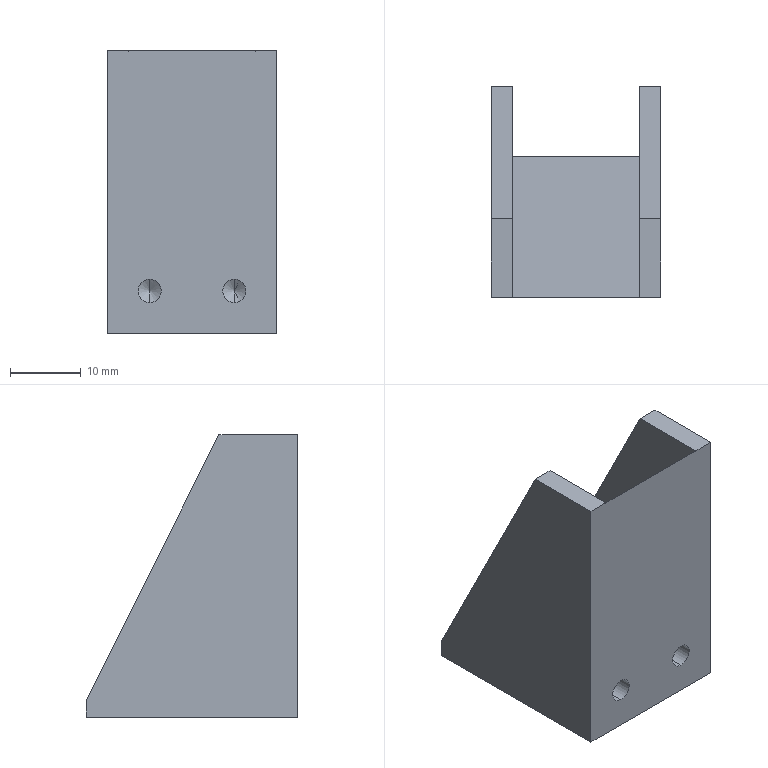Part | STEP file | Discharge hopper | 1 solid | 21 faces | box 24 x 30 x 40 mm | volume 12073 mm3 | plane 13 | cylinder 4 | cone 4 | commonest cylinder face diameters 3.3 x4
STEP:
#1=CARTESIAN_POINT('',(0.,0.,0.));
#2=DIRECTION('',(0.,0.,1.));
#3=DIRECTION('',(1.,0.,0.));
#4=AXIS2_PLACEMENT_3D('',#1,#2,#3);
#5=CARTESIAN_POINT('',(18.,11.5,4.35));
#6=VERTEX_POINT('',#5);
#7=CARTESIAN_POINT('',(18.,0.,4.35));
#8=VERTEX_POINT('',#7);
#9=CARTESIAN_POINT('',(18.,0.,4.35));
#10=DIRECTION('',(0.,-1.,0.));
#11=VECTOR('',#10,1.);
#12=LINE('',#9,#11);
#13=CARTESIAN_POINT('',(18.,0.,6.));
#14=DIRECTION('',(0.,-1.,0.));
#15=DIRECTION('',(0.,0.,-1.));
#16=AXIS2_PLACEMENT_3D('',#13,#14,#15);
#17=CYLINDRICAL_SURFACE('',#16,1.65);
#18=CARTESIAN_POINT('',(6.283,0.));
#19=DIRECTION('',(0.,1.));
#20=VECTOR('',#19,1.);
#21=LINE('',#18,#20);
#22=(GEOMETRIC_REPRESENTATION_CONTEXT(2)PARAMETRIC_REPRESENTATION_CONTEXT()REPRESENTATION_CONTEXT('',''));
#23=DEFINITIONAL_REPRESENTATION('',(#21),#22);
#24=PCURVE('',#17,#23);
#25=CARTESIAN_POINT('',(18.,0.,6.));
#26=DIRECTION('',(0.,-1.,0.));
#27=DIRECTION('',(0.,0.,-1.));
#28=AXIS2_PLACEMENT_3D('',#25,#26,#27);
#29=CYLINDRICAL_SURFACE('',#28,1.65);
#30=CARTESIAN_POINT('',(0.,0.));
#31=DIRECTION('',(0.,1.));
#32=VECTOR('',#31,1.);
#33=LINE('',#30,#32);
#34=(GEOMETRIC_REPRESENTATION_CONTEXT(2)PARAMETRIC_REPRESENTATION_CONTEXT()REPRESENTATION_CONTEXT('',''));
#35=DEFINITIONAL_REPRESENTATION('',(#33),#34);
#36=PCURVE('',#29,#35);
#37=SURFACE_CURVE('',#12,(#24,#36),.PCURVE_S1.);
#38=EDGE_CURVE('',#6,#8,#37,.T.);
#39=ORIENTED_EDGE('',*,*,#38,.T.);
#40=CARTESIAN_POINT('',(18.,0.,7.65));
#41=VERTEX_POINT('',#40);
#42=CARTESIAN_POINT('',(18.,0.,6.));
#43=DIRECTION('',(0.,-1.,0.));
#44=DIRECTION('',(0.,0.,-1.));
#45=AXIS2_PLACEMENT_3D('',#42,#43,#44);
#46=CIRCLE('',#45,1.65);
#47=CARTESIAN_POINT('',(0.,0.));
#48=DIRECTION('',(1.,0.));
#49=VECTOR('',#48,1.);
#50=LINE('',#47,#49);
#51=(GEOMETRIC_REPRESENTATION_CONTEXT(2)PARAMETRIC_REPRESENTATION_CONTEXT()REPRESENTATION_CONTEXT('',''));
#52=DEFINITIONAL_REPRESENTATION('',(#50),#51);
#53=PCURVE('',#17,#52);
#54=CARTESIAN_POINT('',(0.,0.,40.));
#55=DIRECTION('',(0.,1.,0.));
#56=DIRECTION('',(0.,0.,1.));
#57=AXIS2_PLACEMENT_3D('',#54,#55,#56);
#58=PLANE('',#57);
#59=CARTESIAN_POINT('',(-35.65,18.));
#60=CARTESIAN_POINT('',(-35.65,20.858));
#61=CARTESIAN_POINT('',(-33.175,19.429));
#62=CARTESIAN_POINT('',(-30.7,18.));
#63=CARTESIAN_POINT('',(-33.175,16.571));
#64=CARTESIAN_POINT('',(-35.65,15.142));
#65=CARTESIAN_POINT('',(-35.65,18.));
#66=(BOUNDED_CURVE()B_SPLINE_CURVE(2,(#59,#60,#61,#62,#63,#64,#65),.UNSPECIFIED.,.T.,.F.)B_SPLINE_CURVE_WITH_KNOTS((1,2,2,2,2,1),(-2.094,0.,2.094,4.189,6.283,8.378),.UNSPECIFIED.)CURVE()GEOMETRIC_REPRESENTATION_ITEM()RATIONAL_B_SPLINE_CURVE((1.,0.5,1.,0.5,1.,0.5,1.))REPRESENTATION_ITEM(''));
#67=(GEOMETRIC_REPRESENTATION_CONTEXT(2)PARAMETRIC_REPRESENTATION_CONTEXT()REPRESENTATION_CONTEXT('',''));
#68=DEFINITIONAL_REPRESENTATION('',(#66),#67);
#69=PCURVE('',#58,#68);
#70=SURFACE_CURVE('',#46,(#53,#69),.PCURVE_S1.);
#71=EDGE_CURVE('',#41,#8,#70,.T.);
#72=ORIENTED_EDGE('',*,*,#71,.F.);
#73=CARTESIAN_POINT('',(18.,11.5,7.65));
#74=VERTEX_POINT('',#73);
#75=CARTESIAN_POINT('',(18.,0.,7.65));
#76=DIRECTION('',(0.,-1.,0.));
#77=VECTOR('',#76,1.);
#78=LINE('',#75,#77);
#79=CARTESIAN_POINT('',(3.142,0.));
#80=DIRECTION('',(0.,1.));
#81=VECTOR('',#80,1.);
#82=LINE('',#79,#81);
#83=(GEOMETRIC_REPRESENTATION_CONTEXT(2)PARAMETRIC_REPRESENTATION_CONTEXT()REPRESENTATION_CONTEXT('',''));
#84=DEFINITIONAL_REPRESENTATION('',(#82),#83);
#85=PCURVE('',#17,#84);
#86=CARTESIAN_POINT('',(3.142,0.));
#87=DIRECTION('',(0.,1.));
#88=VECTOR('',#87,1.);
#89=LINE('',#86,#88);
#90=(GEOMETRIC_REPRESENTATION_CONTEXT(2)PARAMETRIC_REPRESENTATION_CONTEXT()REPRESENTATION_CONTEXT('',''));
#91=DEFINITIONAL_REPRESENTATION('',(#89),#90);
#92=PCURVE('',#29,#91);
#93=SURFACE_CURVE('',#78,(#85,#92),.PCURVE_S1.);
#94=EDGE_CURVE('',#74,#41,#93,.T.);
#95=ORIENTED_EDGE('',*,*,#94,.F.);
#96=CARTESIAN_POINT('',(18.,11.5,6.));
#97=DIRECTION('',(0.,-1.,0.));
#98=DIRECTION('',(0.,0.,-1.));
#99=AXIS2_PLACEMENT_3D('',#96,#97,#98);
#100=CIRCLE('',#99,1.65);
#101=CARTESIAN_POINT('',(0.,-11.5));
#102=DIRECTION('',(1.,0.));
#103=VECTOR('',#102,1.);
#104=LINE('',#101,#103);
#105=(GEOMETRIC_REPRESENTATION_CONTEXT(2)PARAMETRIC_REPRESENTATION_CONTEXT()REPRESENTATION_CONTEXT('',''));
#106=DEFINITIONAL_REPRESENTATION('',(#104),#105);
#107=PCURVE('',#17,#106);
#108=CARTESIAN_POINT('',(18.,11.5,6.));
#109=DIRECTION('',(0.,-1.,0.));
#110=DIRECTION('',(0.,0.,-1.));
#111=AXIS2_PLACEMENT_3D('',#108,#109,#110);
#112=CONICAL_SURFACE('',#111,1.65,1.03);
#113=CARTESIAN_POINT('',(0.,0.));
#114=DIRECTION('',(1.,0.));
#115=VECTOR('',#114,1.);
#116=LINE('',#113,#115);
#117=(GEOMETRIC_REPRESENTATION_CONTEXT(2)PARAMETRIC_REPRESENTATION_CONTEXT()REPRESENTATION_CONTEXT('',''));
#118=DEFINITIONAL_REPRESENTATION('',(#116),#117);
#119=PCURVE('',#112,#118);
#120=SURFACE_CURVE('',#100,(#107,#119),.PCURVE_S1.);
#121=EDGE_CURVE('',#74,#6,#120,.T.);
#122=ORIENTED_EDGE('',*,*,#121,.T.);
#123=EDGE_LOOP('',(#39,#72,#95,#122));
#124=FACE_BOUND('',#123,.F.);
#125=ADVANCED_FACE('',(#124),#17,.F.);
#126=ORIENTED_EDGE('',*,*,#121,.F.);
#127=CARTESIAN_POINT('',(18.,12.491,6.));
#128=VERTEX_POINT('',#127);
#129=CARTESIAN_POINT('',(18.,11.5,7.65));
#130=DIRECTION('',(0.,-0.515,0.8572));
#131=VECTOR('',#130,1.);
#132=LINE('',#129,#131);
#133=CARTESIAN_POINT('',(3.142,0.));
#134=DIRECTION('',(0.,1.));
#135=VECTOR('',#134,1.);
#136=LINE('',#133,#135);
#137=(GEOMETRIC_REPRESENTATION_CONTEXT(2)PARAMETRIC_REPRESENTATION_CONTEXT()REPRESENTATION_CONTEXT('',''));
#138=DEFINITIONAL_REPRESENTATION('',(#136),#137);
#139=PCURVE('',#112,#138);
#140=CARTESIAN_POINT('',(18.,11.5,6.));
#141=DIRECTION('',(0.,-1.,0.));
#142=DIRECTION('',(0.,0.,-1.));
#143=AXIS2_PLACEMENT_3D('',#140,#141,#142);
#144=CONICAL_SURFACE('',#143,1.65,1.03);
#145=CARTESIAN_POINT('',(3.142,0.));
#146=DIRECTION('',(0.,1.));
#147=VECTOR('',#146,1.);
#148=LINE('',#145,#147);
#149=(GEOMETRIC_REPRESENTATION_CONTEXT(2)PARAMETRIC_REPRESENTATION_CONTEXT()REPRESENTATION_CONTEXT('',''));
#150=DEFINITIONAL_REPRESENTATION('',(#148),#149);
#151=PCURVE('',#144,#150);
#152=SURFACE_CURVE('',#132,(#139,#151),.PCURVE_S1.);
#153=EDGE_CURVE('',#128,#74,#152,.T.);
#154=ORIENTED_EDGE('',*,*,#153,.F.);
#155=CARTESIAN_POINT('',(18.,11.5,4.35));
#156=DIRECTION('',(0.,-0.515,-0.8572));
#157=VECTOR('',#156,1.);
#158=LINE('',#155,#157);
#159=CARTESIAN_POINT('',(6.283,0.));
#160=DIRECTION('',(0.,1.));
#161=VECTOR('',#160,1.);
#162=LINE('',#159,#161);
#163=(GEOMETRIC_REPRESENTATION_CONTEXT(2)PARAMETRIC_REPRESENTATION_CONTEXT()REPRESENTATION_CONTEXT('',''));
#164=DEFINITIONAL_REPRESENTATION('',(#162),#163);
#165=PCURVE('',#112,#164);
#166=CARTESIAN_POINT('',(0.,0.));
#167=DIRECTION('',(0.,1.));
#168=VECTOR('',#167,1.);
#169=LINE('',#166,#168);
#170=(GEOMETRIC_REPRESENTATION_CONTEXT(2)PARAMETRIC_REPRESENTATION_CONTEXT()REPRESENTATION_CONTEXT('',''));
#171=DEFINITIONAL_REPRESENTATION('',(#169),#170);
#172=PCURVE('',#144,#171);
#173=SURFACE_CURVE('',#158,(#165,#172),.PCURVE_S1.);
#174=EDGE_CURVE('',#128,#6,#173,.T.);
#175=ORIENTED_EDGE('',*,*,#174,.T.);
#176=EDGE_LOOP('',(#126,#154,#175));
#177=FACE_BOUND('',#176,.F.);
#178=ADVANCED_FACE('',(#177),#112,.F.);
#179=CARTESIAN_POINT('',(6.,11.5,4.35));
#180=VERTEX_POINT('',#179);
#181=CARTESIAN_POINT('',(6.,0.,4.35));
#182=VERTEX_POINT('',#181);
#183=CARTESIAN_POINT('',(6.,0.,4.35));
#184=DIRECTION('',(0.,-1.,0.));
#185=VECTOR('',#184,1.);
#186=LINE('',#183,#185);
#187=CARTESIAN_POINT('',(6.,0.,6.));
#188=DIRECTION('',(0.,-1.,0.));
#189=DIRECTION('',(0.,0.,-1.));
#190=AXIS2_PLACEMENT_3D('',#187,#188,#189);
#191=CYLINDRICAL_SURFACE('',#190,1.65);
#192=CARTESIAN_POINT('',(6.283,0.));
#193=DIRECTION('',(0.,1.));
#194=VECTOR('',#193,1.);
#195=LINE('',#192,#194);
#196=(GEOMETRIC_REPRESENTATION_CONTEXT(2)PARAMETRIC_REPRESENTATION_CONTEXT()REPRESENTATION_CONTEXT('',''));
#197=DEFINITIONAL_REPRESENTATION('',(#195),#196);
#198=PCURVE('',#191,#197);
#199=CARTESIAN_POINT('',(6.,0.,6.));
#200=DIRECTION('',(0.,-1.,0.));
#201=DIRECTION('',(0.,0.,-1.));
#202=AXIS2_PLACEMENT_3D('',#199,#200,#201);
#203=CYLINDRICAL_SURFACE('',#202,1.65);
#204=CARTESIAN_POINT('',(0.,0.));
#205=DIRECTION('',(0.,1.));
#206=VECTOR('',#205,1.);
#207=LINE('',#204,#206);
#208=(GEOMETRIC_REPRESENTATION_CONTEXT(2)PARAMETRIC_REPRESENTATION_CONTEXT()REPRESENTATION_CONTEXT('',''));
#209=DEFINITIONAL_REPRESENTATION('',(#207),#208);
#210=PCURVE('',#203,#209);
#211=SURFACE_CURVE('',#186,(#198,#210),.PCURVE_S1.);
#212=EDGE_CURVE('',#180,#182,#211,.T.);
#213=ORIENTED_EDGE('',*,*,#212,.T.);
#214=CARTESIAN_POINT('',(6.,0.,7.65));
#215=VERTEX_POINT('',#214);
#216=CARTESIAN_POINT('',(6.,0.,6.));
#217=DIRECTION('',(0.,-1.,0.));
#218=DIRECTION('',(0.,0.,-1.));
#219=AXIS2_PLACEMENT_3D('',#216,#217,#218);
#220=CIRCLE('',#219,1.65);
#221=CARTESIAN_POINT('',(0.,0.));
#222=DIRECTION('',(1.,0.));
#223=VECTOR('',#222,1.);
#224=LINE('',#221,#223);
#225=(GEOMETRIC_REPRESENTATION_CONTEXT(2)PARAMETRIC_REPRESENTATION_CONTEXT()REPRESENTATION_CONTEXT('',''));
#226=DEFINITIONAL_REPRESENTATION('',(#224),#225);
#227=PCURVE('',#191,#226);
#228=CARTESIAN_POINT('',(-35.65,6.));
#229=CARTESIAN_POINT('',(-35.65,8.858));
#230=CARTESIAN_POINT('',(-33.175,7.429));
#231=CARTESIAN_POINT('',(-30.7,6.));
#232=CARTESIAN_POINT('',(-33.175,4.571));
#233=CARTESIAN_POINT('',(-35.65,3.142));
#234=CARTESIAN_POINT('',(-35.65,6.));
#235=(BOUNDED_CURVE()B_SPLINE_CURVE(2,(#228,#229,#230,#231,#232,#233,#234),.UNSPECIFIED.,.T.,.F.)B_SPLINE_CURVE_WITH_KNOTS((1,2,2,2,2,1),(-2.094,0.,2.094,4.189,6.283,8.378),.UNSPECIFIED.)CURVE()GEOMETRIC_REPRESENTATION_ITEM()RATIONAL_B_SPLINE_CURVE((1.,0.5,1.,0.5,1.,0.5,1.))REPRESENTATION_ITEM(''));
#236=(GEOMETRIC_REPRESENTATION_CONTEXT(2)PARAMETRIC_REPRESENTATION_CONTEXT()REPRESENTATION_CONTEXT('',''));
#237=DEFINITIONAL_REPRESENTATION('',(#235),#236);
#238=PCURVE('',#58,#237);
#239=SURFACE_CURVE('',#220,(#227,#238),.PCURVE_S1.);
#240=EDGE_CURVE('',#215,#182,#239,.T.);
#241=ORIENTED_EDGE('',*,*,#240,.F.);
#242=CARTESIAN_POINT('',(6.,11.5,7.65));
#243=VERTEX_POINT('',#242);
#244=CARTESIAN_POINT('',(6.,0.,7.65));
#245=DIRECTION('',(0.,-1.,0.));
#246=VECTOR('',#245,1.);
#247=LINE('',#244,#246);
#248=CARTESIAN_POINT('',(3.142,0.));
#249=DIRECTION('',(0.,1.));
#250=VECTOR('',#249,1.);
#251=LINE('',#248,#250);
#252=(GEOMETRIC_REPRESENTATION_CONTEXT(2)PARAMETRIC_REPRESENTATION_CONTEXT()REPRESENTATION_CONTEXT('',''));
#253=DEFINITIONAL_REPRESENTATION('',(#251),#252);
#254=PCURVE('',#191,#253);
#255=CARTESIAN_POINT('',(3.142,0.));
#256=DIRECTION('',(0.,1.));
#257=VECTOR('',#256,1.);
#258=LINE('',#255,#257);
#259=(GEOMETRIC_REPRESENTATION_CONTEXT(2)PARAMETRIC_REPRESENTATION_CONTEXT()REPRESENTATION_CONTEXT('',''));
#260=DEFINITIONAL_REPRESENTATION('',(#258),#259);
#261=PCURVE('',#203,#260);
#262=SURFACE_CURVE('',#247,(#254,#261),.PCURVE_S1.);
#263=EDGE_CURVE('',#243,#215,#262,.T.);
#264=ORIENTED_EDGE('',*,*,#263,.F.);
#265=CARTESIAN_POINT('',(6.,11.5,6.));
#266=DIRECTION('',(0.,-1.,0.));
#267=DIRECTION('',(0.,0.,-1.));
#268=AXIS2_PLACEMENT_3D('',#265,#266,#267);
#269=CIRCLE('',#268,1.65);
#270=CARTESIAN_POINT('',(0.,-11.5));
#271=DIRECTION('',(1.,0.));
#272=VECTOR('',#271,1.);
#273=LINE('',#270,#272);
#274=(GEOMETRIC_REPRESENTATION_CONTEXT(2)PARAMETRIC_REPRESENTATION_CONTEXT()REPRESENTATION_CONTEXT('',''));
#275=DEFINITIONAL_REPRESENTATION('',(#273),#274);
#276=PCURVE('',#191,#275);
#277=CARTESIAN_POINT('',(6.,11.5,6.));
#278=DIRECTION('',(0.,-1.,0.));
#279=DIRECTION('',(0.,0.,-1.));
#280=AXIS2_PLACEMENT_3D('',#277,#278,#279);
#281=CONICAL_SURFACE('',#280,1.65,1.03);
#282=CARTESIAN_POINT('',(0.,0.));
#283=DIRECTION('',(1.,0.));
#284=VECTOR('',#283,1.);
#285=LINE('',#282,#284);
#286=(GEOMETRIC_REPRESENTATION_CONTEXT(2)PARAMETRIC_REPRESENTATION_CONTEXT()REPRESENTATION_CONTEXT('',''));
#287=DEFINITIONAL_REPRESENTATION('',(#285),#286);
#288=PCURVE('',#281,#287);
#289=SURFACE_CURVE('',#269,(#276,#288),.PCURVE_S1.);
#290=EDGE_CURVE('',#243,#180,#289,.T.);
#291=ORIENTED_EDGE('',*,*,#290,.T.);
#292=EDGE_LOOP('',(#213,#241,#264,#291));
#293=FACE_BOUND('',#292,.F.);
#294=ADVANCED_FACE('',(#293),#191,.F.);
#295=ORIENTED_EDGE('',*,*,#290,.F.);
#296=CARTESIAN_POINT('',(6.,12.491,6.));
#297=VERTEX_POINT('',#296);
#298=CARTESIAN_POINT('',(6.,11.5,7.65));
#299=DIRECTION('',(0.,-0.515,0.8572));
#300=VECTOR('',#299,1.);
#301=LINE('',#298,#300);
#302=CARTESIAN_POINT('',(3.142,0.));
#303=DIRECTION('',(0.,1.));
#304=VECTOR('',#303,1.);
#305=LINE('',#302,#304);
#306=(GEOMETRIC_REPRESENTATION_CONTEXT(2)PARAMETRIC_REPRESENTATION_CONTEXT()REPRESENTATION_CONTEXT('',''));
#307=DEFINITIONAL_REPRESENTATION('',(#305),#306);
#308=PCURVE('',#281,#307);
#309=CARTESIAN_POINT('',(6.,11.5,6.));
#310=DIRECTION('',(0.,-1.,0.));
#311=DIRECTION('',(0.,0.,-1.));
#312=AXIS2_PLACEMENT_3D('',#309,#310,#311);
#313=CONICAL_SURFACE('',#312,1.65,1.03);
#314=CARTESIAN_POINT('',(3.142,0.));
#315=DIRECTION('',(0.,1.));
#316=VECTOR('',#315,1.);
#317=LINE('',#314,#316);
#318=(GEOMETRIC_REPRESENTATION_CONTEXT(2)PARAMETRIC_REPRESENTATION_CONTEXT()REPRESENTATION_CONTEXT('',''));
#319=DEFINITIONAL_REPRESENTATION('',(#317),#318);
#320=PCURVE('',#313,#319);
#321=SURFACE_CURVE('',#301,(#308,#320),.PCURVE_S1.);
#322=EDGE_CURVE('',#297,#243,#321,.T.);
#323=ORIENTED_EDGE('',*,*,#322,.F.);
#324=CARTESIAN_POINT('',(6.,11.5,4.35));
#325=DIRECTION('',(0.,-0.515,-0.8572));
#326=VECTOR('',#325,1.);
#327=LINE('',#324,#326);
#328=CARTESIAN_POINT('',(6.283,0.));
#329=DIRECTION('',(0.,1.));
#330=VECTOR('',#329,1.);
#331=LINE('',#328,#330);
#332=(GEOMETRIC_REPRESENTATION_CONTEXT(2)PARAMETRIC_REPRESENTATION_CONTEXT()REPRESENTATION_CONTEXT('',''));
#333=DEFINITIONAL_REPRESENTATION('',(#331),#332);
#334=PCURVE('',#281,#333);
#335=CARTESIAN_POINT('',(0.,0.));
#336=DIRECTION('',(0.,1.));
#337=VECTOR('',#336,1.);
#338=LINE('',#335,#337);
#339=(GEOMETRIC_REPRESENTATION_CONTEXT(2)PARAMETRIC_REPRESENTATION_CONTEXT()REPRESENTATION_CONTEXT('',''));
#340=DEFINITIONAL_REPRESENTATION('',(#338),#339);
#341=PCURVE('',#313,#340);
#342=SURFACE_CURVE('',#327,(#334,#341),.PCURVE_S1.);
#343=EDGE_CURVE('',#297,#180,#342,.T.);
#344=ORIENTED_EDGE('',*,*,#343,.T.);
#345=EDGE_LOOP('',(#295,#323,#344));
#346=FACE_BOUND('',#345,.F.);
#347=ADVANCED_FACE('',(#346),#281,.F.);
#348=CARTESIAN_POINT('',(21.,30.,2.361));
#349=VERTEX_POINT('',#348);
#350=CARTESIAN_POINT('',(21.,30.,0.));
#351=VERTEX_POINT('',#350);
#352=CARTESIAN_POINT('',(21.,30.,40.));
#353=DIRECTION('',(0.,0.,-1.));
#354=VECTOR('',#353,1.);
#355=LINE('',#352,#354);
#356=CARTESIAN_POINT('',(0.,30.,40.));
#357=DIRECTION('',(0.,-1.,0.));
#358=DIRECTION('',(0.,0.,-1.));
#359=AXIS2_PLACEMENT_3D('',#356,#357,#358);
#360=PLANE('',#359);
#361=CARTESIAN_POINT('',(0.,21.));
#362=DIRECTION('',(1.,0.));
#363=VECTOR('',#362,1.);
#364=LINE('',#361,#363);
#365=(GEOMETRIC_REPRESENTATION_CONTEXT(2)PARAMETRIC_REPRESENTATION_CONTEXT()REPRESENTATION_CONTEXT('',''));
#366=DEFINITIONAL_REPRESENTATION('',(#364),#365);
#367=PCURVE('',#360,#366);
#368=CARTESIAN_POINT('',(21.,0.,44.954));
#369=DIRECTION('',(-1.,0.,0.));
#370=DIRECTION('',(0.,-1.,0.));
#371=AXIS2_PLACEMENT_3D('',#368,#369,#370);
#372=PLANE('',#371);
#373=CARTESIAN_POINT('',(-30.,-4.954));
#374=DIRECTION('',(0.,-1.));
#375=VECTOR('',#374,1.);
#376=LINE('',#373,#375);
#377=(GEOMETRIC_REPRESENTATION_CONTEXT(2)PARAMETRIC_REPRESENTATION_CONTEXT()REPRESENTATION_CONTEXT('',''));
#378=DEFINITIONAL_REPRESENTATION('',(#376),#377);
#379=PCURVE('',#372,#378);
#380=SURFACE_CURVE('',#355,(#367,#379),.PCURVE_S1.);
#381=EDGE_CURVE('',#349,#351,#380,.T.);
#382=ORIENTED_EDGE('',*,*,#381,.F.);
#383=CARTESIAN_POINT('',(24.,30.,2.361));
#384=VERTEX_POINT('',#383);
#385=CARTESIAN_POINT('',(0.,30.,2.361));
#386=DIRECTION('',(1.,0.,0.));
#387=VECTOR('',#386,1.);
#388=LINE('',#385,#387);
#389=CARTESIAN_POINT('',(37.639,0.));
#390=DIRECTION('',(0.,1.));
#391=VECTOR('',#390,1.);
#392=LINE('',#389,#391);
#393=(GEOMETRIC_REPRESENTATION_CONTEXT(2)PARAMETRIC_REPRESENTATION_CONTEXT()REPRESENTATION_CONTEXT('',''));
#394=DEFINITIONAL_REPRESENTATION('',(#392),#393);
#395=PCURVE('',#360,#394);
#396=CARTESIAN_POINT('',(24.,32.456,-2.551));
#397=DIRECTION('',(0.,-0.8944,-0.4472));
#398=DIRECTION('',(0.,0.4472,-0.8944));
#399=AXIS2_PLACEMENT_3D('',#396,#397,#398);
#400=PLANE('',#399);
#401=CARTESIAN_POINT('',(-5.491,-24.));
#402=DIRECTION('',(0.,1.));
#403=VECTOR('',#402,1.);
#404=LINE('',#401,#403);
#405=(GEOMETRIC_REPRESENTATION_CONTEXT(2)PARAMETRIC_REPRESENTATION_CONTEXT()REPRESENTATION_CONTEXT('',''));
#406=DEFINITIONAL_REPRESENTATION('',(#404),#405);
#407=PCURVE('',#400,#406);
#408=SURFACE_CURVE('',#388,(#395,#407),.PCURVE_S1.);
#409=EDGE_CURVE('',#349,#384,#408,.T.);
#410=ORIENTED_EDGE('',*,*,#409,.T.);
#411=CARTESIAN_POINT('',(24.,30.,0.));
#412=VERTEX_POINT('',#411);
#413=CARTESIAN_POINT('',(24.,30.,40.));
#414=DIRECTION('',(0.,0.,-1.));
#415=VECTOR('',#414,1.);
#416=LINE('',#413,#415);
#417=CARTESIAN_POINT('',(0.,24.));
#418=DIRECTION('',(1.,0.));
#419=VECTOR('',#418,1.);
#420=LINE('',#417,#419);
#421=(GEOMETRIC_REPRESENTATION_CONTEXT(2)PARAMETRIC_REPRESENTATION_CONTEXT()REPRESENTATION_CONTEXT('',''));
#422=DEFINITIONAL_REPRESENTATION('',(#420),#421);
#423=PCURVE('',#360,#422);
#424=CARTESIAN_POINT('',(24.,0.,40.));
#425=DIRECTION('',(-1.,0.,0.));
#426=DIRECTION('',(0.,-1.,0.));
#427=AXIS2_PLACEMENT_3D('',#424,#425,#426);
#428=PLANE('',#427);
#429=CARTESIAN_POINT('',(-30.,0.));
#430=DIRECTION('',(0.,-1.));
#431=VECTOR('',#430,1.);
#432=LINE('',#429,#431);
#433=(GEOMETRIC_REPRESENTATION_CONTEXT(2)PARAMETRIC_REPRESENTATION_CONTEXT()REPRESENTATION_CONTEXT('',''));
#434=DEFINITIONAL_REPRESENTATION('',(#432),#433);
#435=PCURVE('',#428,#434);
#436=SURFACE_CURVE('',#416,(#423,#435),.PCURVE_S1.);
#437=EDGE_CURVE('',#384,#412,#436,.T.);
#438=ORIENTED_EDGE('',*,*,#437,.T.);
#439=CARTESIAN_POINT('',(0.,30.,0.));
#440=DIRECTION('',(-1.,0.,0.));
#441=VECTOR('',#440,1.);
#442=LINE('',#439,#441);
#443=CARTESIAN_POINT('',(40.,0.));
#444=DIRECTION('',(0.,-1.));
#445=VECTOR('',#444,1.);
#446=LINE('',#443,#445);
#447=(GEOMETRIC_REPRESENTATION_CONTEXT(2)PARAMETRIC_REPRESENTATION_CONTEXT()REPRESENTATION_CONTEXT('',''));
#448=DEFINITIONAL_REPRESENTATION('',(#446),#447);
#449=PCURVE('',#360,#448);
#450=CARTESIAN_POINT('',(0.,30.,0.));
#451=DIRECTION('',(0.,0.,-1.));
#452=DIRECTION('',(-1.,0.,0.));
#453=AXIS2_PLACEMENT_3D('',#450,#451,#452);
#454=PLANE('',#453);
#455=CARTESIAN_POINT('',(0.,0.));
#456=DIRECTION('',(1.,0.));
#457=VECTOR('',#456,1.);
#458=LINE('',#455,#457);
#459=(GEOMETRIC_REPRESENTATION_CONTEXT(2)PARAMETRIC_REPRESENTATION_CONTEXT()REPRESENTATION_CONTEXT('',''));
#460=DEFINITIONAL_REPRESENTATION('',(#458),#459);
#461=PCURVE('',#454,#460);
#462=SURFACE_CURVE('',#442,(#449,#461),.PCURVE_S1.);
#463=EDGE_CURVE('',#412,#351,#462,.T.);
#464=ORIENTED_EDGE('',*,*,#463,.T.);
#465=EDGE_LOOP('',(#382,#410,#438,#464));
#466=FACE_BOUND('',#465,.T.);
#467=ADVANCED_FACE('',(#466),#360,.F.);
#468=CARTESIAN_POINT('',(24.,0.,40.));
#469=VERTEX_POINT('',#468);
#470=CARTESIAN_POINT('',(24.,11.18,40.));
#471=VERTEX_POINT('',#470);
#472=CARTESIAN_POINT('',(24.,0.,40.));
#473=DIRECTION('',(0.,1.,0.));
#474=VECTOR('',#473,1.);
#475=LINE('',#472,#474);
#476=CARTESIAN_POINT('',(0.,30.,40.));
#477=DIRECTION('',(0.,0.,-1.));
#478=DIRECTION('',(-1.,0.,0.));
#479=AXIS2_PLACEMENT_3D('',#476,#477,#478);
#480=PLANE('',#479);
#481=CARTESIAN_POINT('',(-24.,-30.));
#482=DIRECTION('',(0.,1.));
#483=VECTOR('',#482,1.);
#484=LINE('',#481,#483);
#485=(GEOMETRIC_REPRESENTATION_CONTEXT(2)PARAMETRIC_REPRESENTATION_CONTEXT()REPRESENTATION_CONTEXT('',''));
#486=DEFINITIONAL_REPRESENTATION('',(#484),#485);
#487=PCURVE('',#480,#486);
#488=CARTESIAN_POINT('',(0.,0.));
#489=DIRECTION('',(-1.,0.));
#490=VECTOR('',#489,1.);
#491=LINE('',#488,#490);
#492=(GEOMETRIC_REPRESENTATION_CONTEXT(2)PARAMETRIC_REPRESENTATION_CONTEXT()REPRESENTATION_CONTEXT('',''));
#493=DEFINITIONAL_REPRESENTATION('',(#491),#492);
#494=PCURVE('',#428,#493);
#495=SURFACE_CURVE('',#475,(#487,#494),.PCURVE_S1.);
#496=EDGE_CURVE('',#469,#471,#495,.T.);
#497=ORIENTED_EDGE('',*,*,#496,.T.);
#498=CARTESIAN_POINT('',(21.,11.18,40.));
#499=VERTEX_POINT('',#498);
#500=CARTESIAN_POINT('',(0.,11.18,40.));
#501=DIRECTION('',(-1.,0.,0.));
#502=VECTOR('',#501,1.);
#503=LINE('',#500,#502);
#504=CARTESIAN_POINT('',(0.,-18.82));
#505=DIRECTION('',(1.,0.));
#506=VECTOR('',#505,1.);
#507=LINE('',#504,#506);
#508=(GEOMETRIC_REPRESENTATION_CONTEXT(2)PARAMETRIC_REPRESENTATION_CONTEXT()REPRESENTATION_CONTEXT('',''));
#509=DEFINITIONAL_REPRESENTATION('',(#507),#508);
#510=PCURVE('',#480,#509);
#511=CARTESIAN_POINT('',(-47.574,-24.));
#512=DIRECTION('',(0.,-1.));
#513=VECTOR('',#512,1.);
#514=LINE('',#511,#513);
#515=(GEOMETRIC_REPRESENTATION_CONTEXT(2)PARAMETRIC_REPRESENTATION_CONTEXT()REPRESENTATION_CONTEXT('',''));
#516=DEFINITIONAL_REPRESENTATION('',(#514),#515);
#517=PCURVE('',#400,#516);
#518=SURFACE_CURVE('',#503,(#510,#517),.PCURVE_S1.);
#519=EDGE_CURVE('',#471,#499,#518,.T.);
#520=ORIENTED_EDGE('',*,*,#519,.T.);
#521=CARTESIAN_POINT('',(21.,0.,40.));
#522=VERTEX_POINT('',#521);
#523=CARTESIAN_POINT('',(21.,30.,40.));
#524=DIRECTION('',(0.,1.,0.));
#525=VECTOR('',#524,1.);
#526=LINE('',#523,#525);
#527=CARTESIAN_POINT('',(-21.,0.));
#528=DIRECTION('',(0.,1.));
#529=VECTOR('',#528,1.);
#530=LINE('',#527,#529);
#531=(GEOMETRIC_REPRESENTATION_CONTEXT(2)PARAMETRIC_REPRESENTATION_CONTEXT()REPRESENTATION_CONTEXT('',''));
#532=DEFINITIONAL_REPRESENTATION('',(#530),#531);
#533=PCURVE('',#480,#532);
#534=CARTESIAN_POINT('',(-30.,-4.954));
#535=DIRECTION('',(-1.,0.));
#536=VECTOR('',#535,1.);
#537=LINE('',#534,#536);
#538=(GEOMETRIC_REPRESENTATION_CONTEXT(2)PARAMETRIC_REPRESENTATION_CONTEXT()REPRESENTATION_CONTEXT('',''));
#539=DEFINITIONAL_REPRESENTATION('',(#537),#538);
#540=PCURVE('',#372,#539);
#541=SURFACE_CURVE('',#526,(#533,#540),.PCURVE_S1.);
#542=EDGE_CURVE('',#522,#499,#541,.T.);
#543=ORIENTED_EDGE('',*,*,#542,.F.);
#544=CARTESIAN_POINT('',(0.,0.,40.));
#545=DIRECTION('',(1.,0.,0.));
#546=VECTOR('',#545,1.);
#547=LINE('',#544,#546);
#548=CARTESIAN_POINT('',(0.,-30.));
#549=DIRECTION('',(-1.,0.));
#550=VECTOR('',#549,1.);
#551=LINE('',#548,#550);
#552=(GEOMETRIC_REPRESENTATION_CONTEXT(2)PARAMETRIC_REPRESENTATION_CONTEXT()REPRESENTATION_CONTEXT('',''));
#553=DEFINITIONAL_REPRESENTATION('',(#551),#552);
#554=PCURVE('',#480,#553);
#555=CARTESIAN_POINT('',(0.,0.));
#556=DIRECTION('',(0.,1.));
#557=VECTOR('',#556,1.);
#558=LINE('',#555,#557);
#559=(GEOMETRIC_REPRESENTATION_CONTEXT(2)PARAMETRIC_REPRESENTATION_CONTEXT()REPRESENTATION_CONTEXT('',''));
#560=DEFINITIONAL_REPRESENTATION('',(#558),#559);
#561=PCURVE('',#58,#560);
#562=SURFACE_CURVE('',#547,(#554,#561),.PCURVE_S1.);
#563=EDGE_CURVE('',#522,#469,#562,.T.);
#564=ORIENTED_EDGE('',*,*,#563,.T.);
#565=EDGE_LOOP('',(#497,#520,#543,#564));
#566=FACE_BOUND('',#565,.T.);
#567=ADVANCED_FACE('',(#566),#480,.F.);
#568=CARTESIAN_POINT('',(21.,20.,0.));
#569=VERTEX_POINT('',#568);
#570=CARTESIAN_POINT('',(3.,20.,0.));
#571=VERTEX_POINT('',#570);
#572=CARTESIAN_POINT('',(21.,20.,0.));
#573=DIRECTION('',(-1.,0.,0.));
#574=VECTOR('',#573,1.);
#575=LINE('',#572,#574);
#576=CARTESIAN_POINT('',(-21.,-10.));
#577=DIRECTION('',(1.,0.));
#578=VECTOR('',#577,1.);
#579=LINE('',#576,#578);
#580=(GEOMETRIC_REPRESENTATION_CONTEXT(2)PARAMETRIC_REPRESENTATION_CONTEXT()REPRESENTATION_CONTEXT('',''));
#581=DEFINITIONAL_REPRESENTATION('',(#579),#580);
#582=PCURVE('',#454,#581);
#583=CARTESIAN_POINT('',(21.,20.,0.));
#584=DIRECTION('',(0.,-0.8944,-0.4472));
#585=DIRECTION('',(0.,0.4472,-0.8944));
#586=AXIS2_PLACEMENT_3D('',#583,#584,#585);
#587=PLANE('',#586);
#588=CARTESIAN_POINT('',(0.,0.));
#589=DIRECTION('',(0.,-1.));
#590=VECTOR('',#589,1.);
#591=LINE('',#588,#590);
#592=(GEOMETRIC_REPRESENTATION_CONTEXT(2)PARAMETRIC_REPRESENTATION_CONTEXT()REPRESENTATION_CONTEXT('',''));
#593=DEFINITIONAL_REPRESENTATION('',(#591),#592);
#594=PCURVE('',#587,#593);
#595=SURFACE_CURVE('',#575,(#582,#594),.PCURVE_S1.);
#596=EDGE_CURVE('',#569,#571,#595,.T.);
#597=ORIENTED_EDGE('',*,*,#596,.F.);
#598=CARTESIAN_POINT('',(21.,30.,0.));
#599=DIRECTION('',(0.,1.,0.));
#600=VECTOR('',#599,1.);
#601=LINE('',#598,#600);
#602=CARTESIAN_POINT('',(-21.,0.));
#603=DIRECTION('',(0.,1.));
#604=VECTOR('',#603,1.);
#605=LINE('',#602,#604);
#606=(GEOMETRIC_REPRESENTATION_CONTEXT(2)PARAMETRIC_REPRESENTATION_CONTEXT()REPRESENTATION_CONTEXT('',''));
#607=DEFINITIONAL_REPRESENTATION('',(#605),#606);
#608=PCURVE('',#454,#607);
#609=CARTESIAN_POINT('',(-30.,-44.954));
#610=DIRECTION('',(-1.,0.));
#611=VECTOR('',#610,1.);
#612=LINE('',#609,#611);
#613=(GEOMETRIC_REPRESENTATION_CONTEXT(2)PARAMETRIC_REPRESENTATION_CONTEXT()REPRESENTATION_CONTEXT('',''));
#614=DEFINITIONAL_REPRESENTATION('',(#612),#613);
#615=PCURVE('',#372,#614);
#616=SURFACE_CURVE('',#601,(#608,#615),.PCURVE_S1.);
#617=EDGE_CURVE('',#569,#351,#616,.T.);
#618=ORIENTED_EDGE('',*,*,#617,.T.);
#619=ORIENTED_EDGE('',*,*,#463,.F.);
#620=CARTESIAN_POINT('',(24.,0.,0.));
#621=VERTEX_POINT('',#620);
#622=CARTESIAN_POINT('',(24.,0.,0.));
#623=DIRECTION('',(0.,1.,0.));
#624=VECTOR('',#623,1.);
#625=LINE('',#622,#624);
#626=CARTESIAN_POINT('',(-24.,-30.));
#627=DIRECTION('',(0.,1.));
#628=VECTOR('',#627,1.);
#629=LINE('',#626,#628);
#630=(GEOMETRIC_REPRESENTATION_CONTEXT(2)PARAMETRIC_REPRESENTATION_CONTEXT()REPRESENTATION_CONTEXT('',''));
#631=DEFINITIONAL_REPRESENTATION('',(#629),#630);
#632=PCURVE('',#454,#631);
#633=CARTESIAN_POINT('',(0.,-40.));
#634=DIRECTION('',(-1.,0.));
#635=VECTOR('',#634,1.);
#636=LINE('',#633,#635);
#637=(GEOMETRIC_REPRESENTATION_CONTEXT(2)PARAMETRIC_REPRESENTATION_CONTEXT()REPRESENTATION_CONTEXT('',''));
#638=DEFINITIONAL_REPRESENTATION('',(#636),#637);
#639=PCURVE('',#428,#638);
#640=SURFACE_CURVE('',#625,(#632,#639),.PCURVE_S1.);
#641=EDGE_CURVE('',#621,#412,#640,.T.);
#642=ORIENTED_EDGE('',*,*,#641,.F.);
#643=CARTESIAN_POINT('',(0.,0.,0.));
#644=VERTEX_POINT('',#643);
#645=CARTESIAN_POINT('',(0.,0.,0.));
#646=DIRECTION('',(1.,0.,0.));
#647=VECTOR('',#646,1.);
#648=LINE('',#645,#647);
#649=CARTESIAN_POINT('',(0.,-30.));
#650=DIRECTION('',(-1.,0.));
#651=VECTOR('',#650,1.);
#652=LINE('',#649,#651);
#653=(GEOMETRIC_REPRESENTATION_CONTEXT(2)PARAMETRIC_REPRESENTATION_CONTEXT()REPRESENTATION_CONTEXT('',''));
#654=DEFINITIONAL_REPRESENTATION('',(#652),#653);
#655=PCURVE('',#454,#654);
#656=CARTESIAN_POINT('',(-40.,0.));
#657=DIRECTION('',(0.,1.));
#658=VECTOR('',#657,1.);
#659=LINE('',#656,#658);
#660=(GEOMETRIC_REPRESENTATION_CONTEXT(2)PARAMETRIC_REPRESENTATION_CONTEXT()REPRESENTATION_CONTEXT('',''));
#661=DEFINITIONAL_REPRESENTATION('',(#659),#660);
#662=PCURVE('',#58,#661);
#663=SURFACE_CURVE('',#648,(#655,#662),.PCURVE_S1.);
#664=EDGE_CURVE('',#644,#621,#663,.T.);
#665=ORIENTED_EDGE('',*,*,#664,.F.);
#666=CARTESIAN_POINT('',(0.,30.,0.));
#667=VERTEX_POINT('',#666);
#668=CARTESIAN_POINT('',(0.,0.,0.));
#669=DIRECTION('',(0.,-1.,0.));
#670=VECTOR('',#669,1.);
#671=LINE('',#668,#670);
#672=CARTESIAN_POINT('',(0.,-30.));
#673=DIRECTION('',(0.,-1.));
#674=VECTOR('',#673,1.);
#675=LINE('',#672,#674);
#676=(GEOMETRIC_REPRESENTATION_CONTEXT(2)PARAMETRIC_REPRESENTATION_CONTEXT()REPRESENTATION_CONTEXT('',''));
#677=DEFINITIONAL_REPRESENTATION('',(#675),#676);
#678=PCURVE('',#454,#677);
#679=CARTESIAN_POINT('',(0.,0.,40.));
#680=DIRECTION('',(1.,0.,0.));
#681=DIRECTION('',(0.,1.,0.));
#682=AXIS2_PLACEMENT_3D('',#679,#680,#681);
#683=PLANE('',#682);
#684=CARTESIAN_POINT('',(0.,-40.));
#685=DIRECTION('',(-1.,0.));
#686=VECTOR('',#685,1.);
#687=LINE('',#684,#686);
#688=(GEOMETRIC_REPRESENTATION_CONTEXT(2)PARAMETRIC_REPRESENTATION_CONTEXT()REPRESENTATION_CONTEXT('',''));
#689=DEFINITIONAL_REPRESENTATION('',(#687),#688);
#690=PCURVE('',#683,#689);
#691=SURFACE_CURVE('',#671,(#678,#690),.PCURVE_S1.);
#692=EDGE_CURVE('',#667,#644,#691,.T.);
#693=ORIENTED_EDGE('',*,*,#692,.F.);
#694=CARTESIAN_POINT('',(3.,30.,0.));
#695=VERTEX_POINT('',#694);
#696=CARTESIAN_POINT('',(0.,30.,0.));
#697=DIRECTION('',(-1.,0.,0.));
#698=VECTOR('',#697,1.);
#699=LINE('',#696,#698);
#700=CARTESIAN_POINT('',(0.,0.));
#701=DIRECTION('',(1.,0.));
#702=VECTOR('',#701,1.);
#703=LINE('',#700,#702);
#704=(GEOMETRIC_REPRESENTATION_CONTEXT(2)PARAMETRIC_REPRESENTATION_CONTEXT()REPRESENTATION_CONTEXT('',''));
#705=DEFINITIONAL_REPRESENTATION('',(#703),#704);
#706=PCURVE('',#454,#705);
#707=CARTESIAN_POINT('',(0.,30.,40.));
#708=DIRECTION('',(0.,-1.,0.));
#709=DIRECTION('',(0.,0.,-1.));
#710=AXIS2_PLACEMENT_3D('',#707,#708,#709);
#711=PLANE('',#710);
#712=CARTESIAN_POINT('',(40.,0.));
#713=DIRECTION('',(0.,-1.));
#714=VECTOR('',#713,1.);
#715=LINE('',#712,#714);
#716=(GEOMETRIC_REPRESENTATION_CONTEXT(2)PARAMETRIC_REPRESENTATION_CONTEXT()REPRESENTATION_CONTEXT('',''));
#717=DEFINITIONAL_REPRESENTATION('',(#715),#716);
#718=PCURVE('',#711,#717);
#719=SURFACE_CURVE('',#699,(#706,#718),.PCURVE_S1.);
#720=EDGE_CURVE('',#695,#667,#719,.T.);
#721=ORIENTED_EDGE('',*,*,#720,.F.);
#722=CARTESIAN_POINT('',(3.,30.,0.));
#723=DIRECTION('',(0.,1.,0.));
#724=VECTOR('',#723,1.);
#725=LINE('',#722,#724);
#726=CARTESIAN_POINT('',(-3.,0.));
#727=DIRECTION('',(0.,1.));
#728=VECTOR('',#727,1.);
#729=LINE('',#726,#728);
#730=(GEOMETRIC_REPRESENTATION_CONTEXT(2)PARAMETRIC_REPRESENTATION_CONTEXT()REPRESENTATION_CONTEXT('',''));
#731=DEFINITIONAL_REPRESENTATION('',(#729),#730);
#732=PCURVE('',#454,#731);
#733=CARTESIAN_POINT('',(3.,0.,44.954));
#734=DIRECTION('',(-1.,0.,0.));
#735=DIRECTION('',(0.,-1.,0.));
#736=AXIS2_PLACEMENT_3D('',#733,#734,#735);
#737=PLANE('',#736);
#738=CARTESIAN_POINT('',(-30.,-44.954));
#739=DIRECTION('',(-1.,0.));
#740=VECTOR('',#739,1.);
#741=LINE('',#738,#740);
#742=(GEOMETRIC_REPRESENTATION_CONTEXT(2)PARAMETRIC_REPRESENTATION_CONTEXT()REPRESENTATION_CONTEXT('',''));
#743=DEFINITIONAL_REPRESENTATION('',(#741),#742);
#744=PCURVE('',#737,#743);
#745=SURFACE_CURVE('',#725,(#732,#744),.PCURVE_S1.);
#746=EDGE_CURVE('',#571,#695,#745,.T.);
#747=ORIENTED_EDGE('',*,*,#746,.F.);
#748=EDGE_LOOP('',(#597,#618,#619,#642,#665,#693,#721,#747));
#749=FACE_BOUND('',#748,.T.);
#750=ADVANCED_FACE('',(#749),#454,.T.);
#751=CARTESIAN_POINT('',(0.,11.18,40.));
#752=VERTEX_POINT('',#751);
#753=CARTESIAN_POINT('',(0.,0.,40.));
#754=VERTEX_POINT('',#753);
#755=CARTESIAN_POINT('',(0.,0.,40.));
#756=DIRECTION('',(0.,-1.,0.));
#757=VECTOR('',#756,1.);
#758=LINE('',#755,#757);
#759=CARTESIAN_POINT('',(0.,0.));
#760=DIRECTION('',(-1.,0.));
#761=VECTOR('',#760,1.);
#762=LINE('',#759,#761);
#763=(GEOMETRIC_REPRESENTATION_CONTEXT(2)PARAMETRIC_REPRESENTATION_CONTEXT()REPRESENTATION_CONTEXT('',''));
#764=DEFINITIONAL_REPRESENTATION('',(#762),#763);
#765=PCURVE('',#683,#764);
#766=CARTESIAN_POINT('',(0.,30.,40.));
#767=DIRECTION('',(0.,0.,-1.));
#768=DIRECTION('',(-1.,0.,0.));
#769=AXIS2_PLACEMENT_3D('',#766,#767,#768);
#770=PLANE('',#769);
#771=CARTESIAN_POINT('',(0.,-30.));
#772=DIRECTION('',(0.,-1.));
#773=VECTOR('',#772,1.);
#774=LINE('',#771,#773);
#775=(GEOMETRIC_REPRESENTATION_CONTEXT(2)PARAMETRIC_REPRESENTATION_CONTEXT()REPRESENTATION_CONTEXT('',''));
#776=DEFINITIONAL_REPRESENTATION('',(#774),#775);
#777=PCURVE('',#770,#776);
#778=SURFACE_CURVE('',#758,(#765,#777),.PCURVE_S1.);
#779=EDGE_CURVE('',#752,#754,#778,.T.);
#780=ORIENTED_EDGE('',*,*,#779,.F.);
#781=CARTESIAN_POINT('',(0.,30.,2.361));
#782=VERTEX_POINT('',#781);
#783=CARTESIAN_POINT('',(0.,32.456,-2.551));
#784=DIRECTION('',(0.,-0.4472,0.8944));
#785=VECTOR('',#784,1.);
#786=LINE('',#783,#785);
#787=CARTESIAN_POINT('',(32.456,-42.551));
#788=DIRECTION('',(-0.4472,0.8944));
#789=VECTOR('',#788,1.);
#790=LINE('',#787,#789);
#791=(GEOMETRIC_REPRESENTATION_CONTEXT(2)PARAMETRIC_REPRESENTATION_CONTEXT()REPRESENTATION_CONTEXT('',''));
#792=DEFINITIONAL_REPRESENTATION('',(#790),#791);
#793=PCURVE('',#683,#792);
#794=CARTESIAN_POINT('',(24.,32.456,-2.551));
#795=DIRECTION('',(0.,-0.8944,-0.4472));
#796=DIRECTION('',(0.,0.4472,-0.8944));
#797=AXIS2_PLACEMENT_3D('',#794,#795,#796);
#798=PLANE('',#797);
#799=CARTESIAN_POINT('',(0.,-24.));
#800=DIRECTION('',(-1.,0.));
#801=VECTOR('',#800,1.);
#802=LINE('',#799,#801);
#803=(GEOMETRIC_REPRESENTATION_CONTEXT(2)PARAMETRIC_REPRESENTATION_CONTEXT()REPRESENTATION_CONTEXT('',''));
#804=DEFINITIONAL_REPRESENTATION('',(#802),#803);
#805=PCURVE('',#798,#804);
#806=SURFACE_CURVE('',#786,(#793,#805),.PCURVE_S1.);
#807=EDGE_CURVE('',#782,#752,#806,.T.);
#808=ORIENTED_EDGE('',*,*,#807,.F.);
#809=CARTESIAN_POINT('',(0.,30.,40.));
#810=DIRECTION('',(0.,0.,-1.));
#811=VECTOR('',#810,1.);
#812=LINE('',#809,#811);
#813=CARTESIAN_POINT('',(30.,0.));
#814=DIRECTION('',(0.,-1.));
#815=VECTOR('',#814,1.);
#816=LINE('',#813,#815);
#817=(GEOMETRIC_REPRESENTATION_CONTEXT(2)PARAMETRIC_REPRESENTATION_CONTEXT()REPRESENTATION_CONTEXT('',''));
#818=DEFINITIONAL_REPRESENTATION('',(#816),#817);
#819=PCURVE('',#683,#818);
#820=CARTESIAN_POINT('',(0.,0.));
#821=DIRECTION('',(1.,0.));
#822=VECTOR('',#821,1.);
#823=LINE('',#820,#822);
#824=(GEOMETRIC_REPRESENTATION_CONTEXT(2)PARAMETRIC_REPRESENTATION_CONTEXT()REPRESENTATION_CONTEXT('',''));
#825=DEFINITIONAL_REPRESENTATION('',(#823),#824);
#826=PCURVE('',#711,#825);
#827=SURFACE_CURVE('',#812,(#819,#826),.PCURVE_S1.);
#828=EDGE_CURVE('',#782,#667,#827,.T.);
#829=ORIENTED_EDGE('',*,*,#828,.T.);
#830=ORIENTED_EDGE('',*,*,#692,.T.);
#831=CARTESIAN_POINT('',(0.,0.,40.));
#832=DIRECTION('',(0.,0.,-1.));
#833=VECTOR('',#832,1.);
#834=LINE('',#831,#833);
#835=CARTESIAN_POINT('',(0.,0.));
#836=DIRECTION('',(0.,-1.));
#837=VECTOR('',#836,1.);
#838=LINE('',#835,#837);
#839=(GEOMETRIC_REPRESENTATION_CONTEXT(2)PARAMETRIC_REPRESENTATION_CONTEXT()REPRESENTATION_CONTEXT('',''));
#840=DEFINITIONAL_REPRESENTATION('',(#838),#839);
#841=PCURVE('',#683,#840);
#842=CARTESIAN_POINT('',(0.,0.));
#843=DIRECTION('',(-1.,0.));
#844=VECTOR('',#843,1.);
#845=LINE('',#842,#844);
#846=(GEOMETRIC_REPRESENTATION_CONTEXT(2)PARAMETRIC_REPRESENTATION_CONTEXT()REPRESENTATION_CONTEXT('',''));
#847=DEFINITIONAL_REPRESENTATION('',(#845),#846);
#848=PCURVE('',#58,#847);
#849=SURFACE_CURVE('',#834,(#841,#848),.PCURVE_S1.);
#850=EDGE_CURVE('',#754,#644,#849,.T.);
#851=ORIENTED_EDGE('',*,*,#850,.F.);
#852=EDGE_LOOP('',(#780,#808,#829,#830,#851));
#853=FACE_BOUND('',#852,.T.);
#854=ADVANCED_FACE('',(#853),#683,.F.);
#855=CARTESIAN_POINT('',(18.,0.,6.));
#856=DIRECTION('',(0.,-1.,0.));
#857=DIRECTION('',(0.,0.,-1.));
#858=AXIS2_PLACEMENT_3D('',#855,#856,#857);
#859=CIRCLE('',#858,1.65);
#860=CARTESIAN_POINT('',(-35.65,18.));
#861=CARTESIAN_POINT('',(-35.65,20.858));
#862=CARTESIAN_POINT('',(-33.175,19.429));
#863=CARTESIAN_POINT('',(-30.7,18.));
#864=CARTESIAN_POINT('',(-33.175,16.571));
#865=CARTESIAN_POINT('',(-35.65,15.142));
#866=CARTESIAN_POINT('',(-35.65,18.));
#867=(BOUNDED_CURVE()B_SPLINE_CURVE(2,(#860,#861,#862,#863,#864,#865,#866),.UNSPECIFIED.,.T.,.F.)B_SPLINE_CURVE_WITH_KNOTS((1,2,2,2,2,1),(-2.094,0.,2.094,4.189,6.283,8.378),.UNSPECIFIED.)CURVE()GEOMETRIC_REPRESENTATION_ITEM()RATIONAL_B_SPLINE_CURVE((1.,0.5,1.,0.5,1.,0.5,1.))REPRESENTATION_ITEM(''));
#868=(GEOMETRIC_REPRESENTATION_CONTEXT(2)PARAMETRIC_REPRESENTATION_CONTEXT()REPRESENTATION_CONTEXT('',''));
#869=DEFINITIONAL_REPRESENTATION('',(#867),#868);
#870=PCURVE('',#58,#869);
#871=CARTESIAN_POINT('',(0.,0.));
#872=DIRECTION('',(1.,0.));
#873=VECTOR('',#872,1.);
#874=LINE('',#871,#873);
#875=(GEOMETRIC_REPRESENTATION_CONTEXT(2)PARAMETRIC_REPRESENTATION_CONTEXT()REPRESENTATION_CONTEXT('',''));
#876=DEFINITIONAL_REPRESENTATION('',(#874),#875);
#877=PCURVE('',#29,#876);
#878=SURFACE_CURVE('',#859,(#870,#877),.PCURVE_S1.);
#879=EDGE_CURVE('',#8,#41,#878,.T.);
#880=ORIENTED_EDGE('',*,*,#879,.F.);
#881=ORIENTED_EDGE('',*,*,#71,.F.);
#882=EDGE_LOOP('',(#880,#881));
#883=FACE_BOUND('',#882,.T.);
#884=CARTESIAN_POINT('',(6.,0.,6.));
#885=DIRECTION('',(0.,-1.,0.));
#886=DIRECTION('',(0.,0.,-1.));
#887=AXIS2_PLACEMENT_3D('',#884,#885,#886);
#888=CIRCLE('',#887,1.65);
#889=CARTESIAN_POINT('',(-35.65,6.));
#890=CARTESIAN_POINT('',(-35.65,8.858));
#891=CARTESIAN_POINT('',(-33.175,7.429));
#892=CARTESIAN_POINT('',(-30.7,6.));
#893=CARTESIAN_POINT('',(-33.175,4.571));
#894=CARTESIAN_POINT('',(-35.65,3.142));
#895=CARTESIAN_POINT('',(-35.65,6.));
#896=(BOUNDED_CURVE()B_SPLINE_CURVE(2,(#889,#890,#891,#892,#893,#894,#895),.UNSPECIFIED.,.T.,.F.)B_SPLINE_CURVE_WITH_KNOTS((1,2,2,2,2,1),(-2.094,0.,2.094,4.189,6.283,8.378),.UNSPECIFIED.)CURVE()GEOMETRIC_REPRESENTATION_ITEM()RATIONAL_B_SPLINE_CURVE((1.,0.5,1.,0.5,1.,0.5,1.))REPRESENTATION_ITEM(''));
#897=(GEOMETRIC_REPRESENTATION_CONTEXT(2)PARAMETRIC_REPRESENTATION_CONTEXT()REPRESENTATION_CONTEXT('',''));
#898=DEFINITIONAL_REPRESENTATION('',(#896),#897);
#899=PCURVE('',#58,#898);
#900=CARTESIAN_POINT('',(0.,0.));
#901=DIRECTION('',(1.,0.));
#902=VECTOR('',#901,1.);
#903=LINE('',#900,#902);
#904=(GEOMETRIC_REPRESENTATION_CONTEXT(2)PARAMETRIC_REPRESENTATION_CONTEXT()REPRESENTATION_CONTEXT('',''));
#905=DEFINITIONAL_REPRESENTATION('',(#903),#904);
#906=PCURVE('',#203,#905);
#907=SURFACE_CURVE('',#888,(#899,#906),.PCURVE_S1.);
#908=EDGE_CURVE('',#182,#215,#907,.T.);
#909=ORIENTED_EDGE('',*,*,#908,.F.);
#910=ORIENTED_EDGE('',*,*,#240,.F.);
#911=EDGE_LOOP('',(#909,#910));
#912=FACE_BOUND('',#911,.T.);
#913=ORIENTED_EDGE('',*,*,#664,.T.);
#914=CARTESIAN_POINT('',(24.,0.,40.));
#915=DIRECTION('',(0.,0.,-1.));
#916=VECTOR('',#915,1.);
#917=LINE('',#914,#916);
#918=CARTESIAN_POINT('',(0.,24.));
#919=DIRECTION('',(-1.,0.));
#920=VECTOR('',#919,1.);
#921=LINE('',#918,#920);
#922=(GEOMETRIC_REPRESENTATION_CONTEXT(2)PARAMETRIC_REPRESENTATION_CONTEXT()REPRESENTATION_CONTEXT('',''));
#923=DEFINITIONAL_REPRESENTATION('',(#921),#922);
#924=PCURVE('',#58,#923);
#925=CARTESIAN_POINT('',(0.,0.));
#926=DIRECTION('',(0.,-1.));
#927=VECTOR('',#926,1.);
#928=LINE('',#925,#927);
#929=(GEOMETRIC_REPRESENTATION_CONTEXT(2)PARAMETRIC_REPRESENTATION_CONTEXT()REPRESENTATION_CONTEXT('',''));
#930=DEFINITIONAL_REPRESENTATION('',(#928),#929);
#931=PCURVE('',#428,#930);
#932=SURFACE_CURVE('',#917,(#924,#931),.PCURVE_S1.);
#933=EDGE_CURVE('',#469,#621,#932,.T.);
#934=ORIENTED_EDGE('',*,*,#933,.F.);
#935=ORIENTED_EDGE('',*,*,#563,.F.);
#936=CARTESIAN_POINT('',(3.,0.,40.));
#937=VERTEX_POINT('',#936);
#938=CARTESIAN_POINT('',(21.,0.,40.));
#939=DIRECTION('',(-1.,0.,0.));
#940=VECTOR('',#939,1.);
#941=LINE('',#938,#940);
#942=CARTESIAN_POINT('',(0.,21.));
#943=DIRECTION('',(0.,-1.));
#944=VECTOR('',#943,1.);
#945=LINE('',#942,#944);
#946=(GEOMETRIC_REPRESENTATION_CONTEXT(2)PARAMETRIC_REPRESENTATION_CONTEXT()REPRESENTATION_CONTEXT('',''));
#947=DEFINITIONAL_REPRESENTATION('',(#945),#946);
#948=PCURVE('',#58,#947);
#949=CARTESIAN_POINT('',(-44.721,0.));
#950=DIRECTION('',(0.,-1.));
#951=VECTOR('',#950,1.);
#952=LINE('',#949,#951);
#953=(GEOMETRIC_REPRESENTATION_CONTEXT(2)PARAMETRIC_REPRESENTATION_CONTEXT()REPRESENTATION_CONTEXT('',''));
#954=DEFINITIONAL_REPRESENTATION('',(#952),#953);
#955=PCURVE('',#587,#954);
#956=SURFACE_CURVE('',#941,(#948,#955),.PCURVE_S1.);
#957=EDGE_CURVE('',#522,#937,#956,.T.);
#958=ORIENTED_EDGE('',*,*,#957,.T.);
#959=CARTESIAN_POINT('',(0.,0.,40.));
#960=DIRECTION('',(1.,0.,0.));
#961=VECTOR('',#960,1.);
#962=LINE('',#959,#961);
#963=CARTESIAN_POINT('',(0.,0.));
#964=DIRECTION('',(0.,1.));
#965=VECTOR('',#964,1.);
#966=LINE('',#963,#965);
#967=(GEOMETRIC_REPRESENTATION_CONTEXT(2)PARAMETRIC_REPRESENTATION_CONTEXT()REPRESENTATION_CONTEXT('',''));
#968=DEFINITIONAL_REPRESENTATION('',(#966),#967);
#969=PCURVE('',#58,#968);
#970=CARTESIAN_POINT('',(0.,-30.));
#971=DIRECTION('',(-1.,0.));
#972=VECTOR('',#971,1.);
#973=LINE('',#970,#972);
#974=(GEOMETRIC_REPRESENTATION_CONTEXT(2)PARAMETRIC_REPRESENTATION_CONTEXT()REPRESENTATION_CONTEXT('',''));
#975=DEFINITIONAL_REPRESENTATION('',(#973),#974);
#976=PCURVE('',#770,#975);
#977=SURFACE_CURVE('',#962,(#969,#976),.PCURVE_S1.);
#978=EDGE_CURVE('',#754,#937,#977,.T.);
#979=ORIENTED_EDGE('',*,*,#978,.F.);
#980=ORIENTED_EDGE('',*,*,#850,.T.);
#981=EDGE_LOOP('',(#913,#934,#935,#958,#979,#980));
#982=FACE_BOUND('',#981,.T.);
#983=ADVANCED_FACE('',(#883,#912,#982),#58,.F.);
#984=ORIENTED_EDGE('',*,*,#437,.F.);
#985=CARTESIAN_POINT('',(24.,32.456,-2.551));
#986=DIRECTION('',(0.,-0.4472,0.8944));
#987=VECTOR('',#986,1.);
#988=LINE('',#985,#987);
#989=CARTESIAN_POINT('',(-32.456,-42.551));
#990=DIRECTION('',(0.4472,0.8944));
#991=VECTOR('',#990,1.);
#992=LINE('',#989,#991);
#993=(GEOMETRIC_REPRESENTATION_CONTEXT(2)PARAMETRIC_REPRESENTATION_CONTEXT()REPRESENTATION_CONTEXT('',''));
#994=DEFINITIONAL_REPRESENTATION('',(#992),#993);
#995=PCURVE('',#428,#994);
#996=CARTESIAN_POINT('',(0.,0.));
#997=DIRECTION('',(-1.,0.));
#998=VECTOR('',#997,1.);
#999=LINE('',#996,#998);
#1000=(GEOMETRIC_REPRESENTATION_CONTEXT(2)PARAMETRIC_REPRESENTATION_CONTEXT()REPRESENTATION_CONTEXT('',''));
#1001=DEFINITIONAL_REPRESENTATION('',(#999),#1000);
#1002=PCURVE('',#400,#1001);
#1003=SURFACE_CURVE('',#988,(#995,#1002),.PCURVE_S1.);
#1004=EDGE_CURVE('',#384,#471,#1003,.T.);
#1005=ORIENTED_EDGE('',*,*,#1004,.T.);
#1006=ORIENTED_EDGE('',*,*,#496,.F.);
#1007=ORIENTED_EDGE('',*,*,#933,.T.);
#1008=ORIENTED_EDGE('',*,*,#641,.T.);
#1009=EDGE_LOOP('',(#984,#1005,#1006,#1007,#1008));
#1010=FACE_BOUND('',#1009,.T.);
#1011=ADVANCED_FACE('',(#1010),#428,.F.);
#1012=ORIENTED_EDGE('',*,*,#828,.F.);
#1013=CARTESIAN_POINT('',(3.,30.,2.361));
#1014=VERTEX_POINT('',#1013);
#1015=CARTESIAN_POINT('',(0.,30.,2.361));
#1016=DIRECTION('',(1.,0.,0.));
#1017=VECTOR('',#1016,1.);
#1018=LINE('',#1015,#1017);
#1019=CARTESIAN_POINT('',(37.639,0.));
#1020=DIRECTION('',(0.,1.));
#1021=VECTOR('',#1020,1.);
#1022=LINE('',#1019,#1021);
#1023=(GEOMETRIC_REPRESENTATION_CONTEXT(2)PARAMETRIC_REPRESENTATION_CONTEXT()REPRESENTATION_CONTEXT('',''));
#1024=DEFINITIONAL_REPRESENTATION('',(#1022),#1023);
#1025=PCURVE('',#711,#1024);
#1026=CARTESIAN_POINT('',(-5.491,-24.));
#1027=DIRECTION('',(0.,1.));
#1028=VECTOR('',#1027,1.);
#1029=LINE('',#1026,#1028);
#1030=(GEOMETRIC_REPRESENTATION_CONTEXT(2)PARAMETRIC_REPRESENTATION_CONTEXT()REPRESENTATION_CONTEXT('',''));
#1031=DEFINITIONAL_REPRESENTATION('',(#1029),#1030);
#1032=PCURVE('',#798,#1031);
#1033=SURFACE_CURVE('',#1018,(#1025,#1032),.PCURVE_S1.);
#1034=EDGE_CURVE('',#782,#1014,#1033,.T.);
#1035=ORIENTED_EDGE('',*,*,#1034,.T.);
#1036=CARTESIAN_POINT('',(3.,30.,40.));
#1037=DIRECTION('',(0.,0.,-1.));
#1038=VECTOR('',#1037,1.);
#1039=LINE('',#1036,#1038);
#1040=CARTESIAN_POINT('',(0.,3.));
#1041=DIRECTION('',(1.,0.));
#1042=VECTOR('',#1041,1.);
#1043=LINE('',#1040,#1042);
#1044=(GEOMETRIC_REPRESENTATION_CONTEXT(2)PARAMETRIC_REPRESENTATION_CONTEXT()REPRESENTATION_CONTEXT('',''));
#1045=DEFINITIONAL_REPRESENTATION('',(#1043),#1044);
#1046=PCURVE('',#711,#1045);
#1047=CARTESIAN_POINT('',(-30.,-4.954));
#1048=DIRECTION('',(0.,-1.));
#1049=VECTOR('',#1048,1.);
#1050=LINE('',#1047,#1049);
#1051=(GEOMETRIC_REPRESENTATION_CONTEXT(2)PARAMETRIC_REPRESENTATION_CONTEXT()REPRESENTATION_CONTEXT('',''));
#1052=DEFINITIONAL_REPRESENTATION('',(#1050),#1051);
#1053=PCURVE('',#737,#1052);
#1054=SURFACE_CURVE('',#1039,(#1046,#1053),.PCURVE_S1.);
#1055=EDGE_CURVE('',#1014,#695,#1054,.T.);
#1056=ORIENTED_EDGE('',*,*,#1055,.T.);
#1057=ORIENTED_EDGE('',*,*,#720,.T.);
#1058=EDGE_LOOP('',(#1012,#1035,#1056,#1057));
#1059=FACE_BOUND('',#1058,.T.);
#1060=ADVANCED_FACE('',(#1059),#711,.F.);
#1061=CARTESIAN_POINT('',(3.,11.18,40.));
#1062=VERTEX_POINT('',#1061);
#1063=CARTESIAN_POINT('',(3.,30.,40.));
#1064=DIRECTION('',(0.,1.,0.));
#1065=VECTOR('',#1064,1.);
#1066=LINE('',#1063,#1065);
#1067=CARTESIAN_POINT('',(-3.,0.));
#1068=DIRECTION('',(0.,1.));
#1069=VECTOR('',#1068,1.);
#1070=LINE('',#1067,#1069);
#1071=(GEOMETRIC_REPRESENTATION_CONTEXT(2)PARAMETRIC_REPRESENTATION_CONTEXT()REPRESENTATION_CONTEXT('',''));
#1072=DEFINITIONAL_REPRESENTATION('',(#1070),#1071);
#1073=PCURVE('',#770,#1072);
#1074=CARTESIAN_POINT('',(-30.,-4.954));
#1075=DIRECTION('',(-1.,0.));
#1076=VECTOR('',#1075,1.);
#1077=LINE('',#1074,#1076);
#1078=(GEOMETRIC_REPRESENTATION_CONTEXT(2)PARAMETRIC_REPRESENTATION_CONTEXT()REPRESENTATION_CONTEXT('',''));
#1079=DEFINITIONAL_REPRESENTATION('',(#1077),#1078);
#1080=PCURVE('',#737,#1079);
#1081=SURFACE_CURVE('',#1066,(#1073,#1080),.PCURVE_S1.);
#1082=EDGE_CURVE('',#937,#1062,#1081,.T.);
#1083=ORIENTED_EDGE('',*,*,#1082,.T.);
#1084=CARTESIAN_POINT('',(0.,11.18,40.));
#1085=DIRECTION('',(-1.,0.,0.));
#1086=VECTOR('',#1085,1.);
#1087=LINE('',#1084,#1086);
#1088=CARTESIAN_POINT('',(0.,-18.82));
#1089=DIRECTION('',(1.,0.));
#1090=VECTOR('',#1089,1.);
#1091=LINE('',#1088,#1090);
#1092=(GEOMETRIC_REPRESENTATION_CONTEXT(2)PARAMETRIC_REPRESENTATION_CONTEXT()REPRESENTATION_CONTEXT('',''));
#1093=DEFINITIONAL_REPRESENTATION('',(#1091),#1092);
#1094=PCURVE('',#770,#1093);
#1095=CARTESIAN_POINT('',(-47.574,-24.));
#1096=DIRECTION('',(0.,-1.));
#1097=VECTOR('',#1096,1.);
#1098=LINE('',#1095,#1097);
#1099=(GEOMETRIC_REPRESENTATION_CONTEXT(2)PARAMETRIC_REPRESENTATION_CONTEXT()REPRESENTATION_CONTEXT('',''));
#1100=DEFINITIONAL_REPRESENTATION('',(#1098),#1099);
#1101=PCURVE('',#798,#1100);
#1102=SURFACE_CURVE('',#1087,(#1094,#1101),.PCURVE_S1.);
#1103=EDGE_CURVE('',#1062,#752,#1102,.T.);
#1104=ORIENTED_EDGE('',*,*,#1103,.T.);
#1105=ORIENTED_EDGE('',*,*,#779,.T.);
#1106=ORIENTED_EDGE('',*,*,#978,.T.);
#1107=EDGE_LOOP('',(#1083,#1104,#1105,#1106));
#1108=FACE_BOUND('',#1107,.T.);
#1109=ADVANCED_FACE('',(#1108),#770,.F.);
#1110=CARTESIAN_POINT('',(21.,6.962,48.436));
#1111=DIRECTION('',(0.,-0.4472,0.8944));
#1112=VECTOR('',#1111,1.);
#1113=LINE('',#1110,#1112);
#1114=CARTESIAN_POINT('',(-6.962,3.481));
#1115=DIRECTION('',(0.4472,0.8944));
#1116=VECTOR('',#1115,1.);
#1117=LINE('',#1114,#1116);
#1118=(GEOMETRIC_REPRESENTATION_CONTEXT(2)PARAMETRIC_REPRESENTATION_CONTEXT()REPRESENTATION_CONTEXT('',''));
#1119=DEFINITIONAL_REPRESENTATION('',(#1117),#1118);
#1120=PCURVE('',#372,#1119);
#1121=CARTESIAN_POINT('',(-57.005,-3.));
#1122=DIRECTION('',(-1.,0.));
#1123=VECTOR('',#1122,1.);
#1124=LINE('',#1121,#1123);
#1125=(GEOMETRIC_REPRESENTATION_CONTEXT(2)PARAMETRIC_REPRESENTATION_CONTEXT()REPRESENTATION_CONTEXT('',''));
#1126=DEFINITIONAL_REPRESENTATION('',(#1124),#1125);
#1127=PCURVE('',#400,#1126);
#1128=SURFACE_CURVE('',#1113,(#1120,#1127),.PCURVE_S1.);
#1129=EDGE_CURVE('',#349,#499,#1128,.T.);
#1130=ORIENTED_EDGE('',*,*,#1129,.F.);
#1131=ORIENTED_EDGE('',*,*,#381,.T.);
#1132=ORIENTED_EDGE('',*,*,#617,.F.);
#1133=CARTESIAN_POINT('',(21.,20.,0.));
#1134=DIRECTION('',(0.,-0.4472,0.8944));
#1135=VECTOR('',#1134,1.);
#1136=LINE('',#1133,#1135);
#1137=CARTESIAN_POINT('',(-20.,-44.954));
#1138=DIRECTION('',(0.4472,0.8944));
#1139=VECTOR('',#1138,1.);
#1140=LINE('',#1137,#1139);
#1141=(GEOMETRIC_REPRESENTATION_CONTEXT(2)PARAMETRIC_REPRESENTATION_CONTEXT()REPRESENTATION_CONTEXT('',''));
#1142=DEFINITIONAL_REPRESENTATION('',(#1140),#1141);
#1143=PCURVE('',#372,#1142);
#1144=CARTESIAN_POINT('',(0.,0.));
#1145=DIRECTION('',(-1.,0.));
#1146=VECTOR('',#1145,1.);
#1147=LINE('',#1144,#1146);
#1148=(GEOMETRIC_REPRESENTATION_CONTEXT(2)PARAMETRIC_REPRESENTATION_CONTEXT()REPRESENTATION_CONTEXT('',''));
#1149=DEFINITIONAL_REPRESENTATION('',(#1147),#1148);
#1150=PCURVE('',#587,#1149);
#1151=SURFACE_CURVE('',#1136,(#1143,#1150),.PCURVE_S1.);
#1152=EDGE_CURVE('',#569,#522,#1151,.T.);
#1153=ORIENTED_EDGE('',*,*,#1152,.T.);
#1154=ORIENTED_EDGE('',*,*,#542,.T.);
#1155=EDGE_LOOP('',(#1130,#1131,#1132,#1153,#1154));
#1156=FACE_BOUND('',#1155,.T.);
#1157=ADVANCED_FACE('',(#1156),#372,.T.);
#1158=ORIENTED_EDGE('',*,*,#1055,.F.);
#1159=CARTESIAN_POINT('',(3.,6.962,48.436));
#1160=DIRECTION('',(0.,-0.4472,0.8944));
#1161=VECTOR('',#1160,1.);
#1162=LINE('',#1159,#1161);
#1163=CARTESIAN_POINT('',(-6.962,3.481));
#1164=DIRECTION('',(0.4472,0.8944));
#1165=VECTOR('',#1164,1.);
#1166=LINE('',#1163,#1165);
#1167=(GEOMETRIC_REPRESENTATION_CONTEXT(2)PARAMETRIC_REPRESENTATION_CONTEXT()REPRESENTATION_CONTEXT('',''));
#1168=DEFINITIONAL_REPRESENTATION('',(#1166),#1167);
#1169=PCURVE('',#737,#1168);
#1170=CARTESIAN_POINT('',(-57.005,-21.));
#1171=DIRECTION('',(-1.,0.));
#1172=VECTOR('',#1171,1.);
#1173=LINE('',#1170,#1172);
#1174=(GEOMETRIC_REPRESENTATION_CONTEXT(2)PARAMETRIC_REPRESENTATION_CONTEXT()REPRESENTATION_CONTEXT('',''));
#1175=DEFINITIONAL_REPRESENTATION('',(#1173),#1174);
#1176=PCURVE('',#798,#1175);
#1177=SURFACE_CURVE('',#1162,(#1169,#1176),.PCURVE_S1.);
#1178=EDGE_CURVE('',#1014,#1062,#1177,.T.);
#1179=ORIENTED_EDGE('',*,*,#1178,.T.);
#1180=ORIENTED_EDGE('',*,*,#1082,.F.);
#1181=CARTESIAN_POINT('',(3.,20.,0.));
#1182=DIRECTION('',(0.,-0.4472,0.8944));
#1183=VECTOR('',#1182,1.);
#1184=LINE('',#1181,#1183);
#1185=CARTESIAN_POINT('',(-20.,-44.954));
#1186=DIRECTION('',(0.4472,0.8944));
#1187=VECTOR('',#1186,1.);
#1188=LINE('',#1185,#1187);
#1189=(GEOMETRIC_REPRESENTATION_CONTEXT(2)PARAMETRIC_REPRESENTATION_CONTEXT()REPRESENTATION_CONTEXT('',''));
#1190=DEFINITIONAL_REPRESENTATION('',(#1188),#1189);
#1191=PCURVE('',#737,#1190);
#1192=CARTESIAN_POINT('',(0.,-18.));
#1193=DIRECTION('',(-1.,0.));
#1194=VECTOR('',#1193,1.);
#1195=LINE('',#1192,#1194);
#1196=(GEOMETRIC_REPRESENTATION_CONTEXT(2)PARAMETRIC_REPRESENTATION_CONTEXT()REPRESENTATION_CONTEXT('',''));
#1197=DEFINITIONAL_REPRESENTATION('',(#1195),#1196);
#1198=PCURVE('',#587,#1197);
#1199=SURFACE_CURVE('',#1184,(#1191,#1198),.PCURVE_S1.);
#1200=EDGE_CURVE('',#571,#937,#1199,.T.);
#1201=ORIENTED_EDGE('',*,*,#1200,.F.);
#1202=ORIENTED_EDGE('',*,*,#746,.T.);
#1203=EDGE_LOOP('',(#1158,#1179,#1180,#1201,#1202));
#1204=FACE_BOUND('',#1203,.T.);
#1205=ADVANCED_FACE('',(#1204),#737,.F.);
#1206=ORIENTED_EDGE('',*,*,#1200,.T.);
#1207=ORIENTED_EDGE('',*,*,#957,.F.);
#1208=ORIENTED_EDGE('',*,*,#1152,.F.);
#1209=ORIENTED_EDGE('',*,*,#596,.T.);
#1210=EDGE_LOOP('',(#1206,#1207,#1208,#1209));
#1211=FACE_BOUND('',#1210,.T.);
#1212=ADVANCED_FACE('',(#1211),#587,.F.);
#1213=ORIENTED_EDGE('',*,*,#807,.T.);
#1214=ORIENTED_EDGE('',*,*,#1103,.F.);
#1215=ORIENTED_EDGE('',*,*,#1178,.F.);
#1216=ORIENTED_EDGE('',*,*,#1034,.F.);
#1217=EDGE_LOOP('',(#1213,#1214,#1215,#1216));
#1218=FACE_BOUND('',#1217,.T.);
#1219=ADVANCED_FACE('',(#1218),#798,.F.);
#1220=ORIENTED_EDGE('',*,*,#1129,.T.);
#1221=ORIENTED_EDGE('',*,*,#519,.F.);
#1222=ORIENTED_EDGE('',*,*,#1004,.F.);
#1223=ORIENTED_EDGE('',*,*,#409,.F.);
#1224=EDGE_LOOP('',(#1220,#1221,#1222,#1223));
#1225=FACE_BOUND('',#1224,.T.);
#1226=ADVANCED_FACE('',(#1225),#400,.F.);
#1227=CARTESIAN_POINT('',(6.,11.5,6.));
#1228=DIRECTION('',(0.,-1.,0.));
#1229=DIRECTION('',(0.,0.,-1.));
#1230=AXIS2_PLACEMENT_3D('',#1227,#1228,#1229);
#1231=CIRCLE('',#1230,1.65);
#1232=CARTESIAN_POINT('',(0.,0.));
#1233=DIRECTION('',(1.,0.));
#1234=VECTOR('',#1233,1.);
#1235=LINE('',#1232,#1234);
#1236=(GEOMETRIC_REPRESENTATION_CONTEXT(2)PARAMETRIC_REPRESENTATION_CONTEXT()REPRESENTATION_CONTEXT('',''));
#1237=DEFINITIONAL_REPRESENTATION('',(#1235),#1236);
#1238=PCURVE('',#313,#1237);
#1239=CARTESIAN_POINT('',(0.,-11.5));
#1240=DIRECTION('',(1.,0.));
#1241=VECTOR('',#1240,1.);
#1242=LINE('',#1239,#1241);
#1243=(GEOMETRIC_REPRESENTATION_CONTEXT(2)PARAMETRIC_REPRESENTATION_CONTEXT()REPRESENTATION_CONTEXT('',''));
#1244=DEFINITIONAL_REPRESENTATION('',(#1242),#1243);
#1245=PCURVE('',#203,#1244);
#1246=SURFACE_CURVE('',#1231,(#1238,#1245),.PCURVE_S1.);
#1247=EDGE_CURVE('',#180,#243,#1246,.T.);
#1248=ORIENTED_EDGE('',*,*,#1247,.F.);
#1249=ORIENTED_EDGE('',*,*,#343,.F.);
#1250=ORIENTED_EDGE('',*,*,#322,.T.);
#1251=EDGE_LOOP('',(#1248,#1249,#1250));
#1252=FACE_BOUND('',#1251,.F.);
#1253=ADVANCED_FACE('',(#1252),#313,.F.);
#1254=ORIENTED_EDGE('',*,*,#908,.F.);
#1255=ORIENTED_EDGE('',*,*,#212,.F.);
#1256=ORIENTED_EDGE('',*,*,#1247,.T.);
#1257=ORIENTED_EDGE('',*,*,#263,.T.);
#1258=EDGE_LOOP('',(#1254,#1255,#1256,#1257));
#1259=FACE_BOUND('',#1258,.F.);
#1260=ADVANCED_FACE('',(#1259),#203,.F.);
#1261=CARTESIAN_POINT('',(18.,11.5,6.));
#1262=DIRECTION('',(0.,-1.,0.));
#1263=DIRECTION('',(0.,0.,-1.));
#1264=AXIS2_PLACEMENT_3D('',#1261,#1262,#1263);
#1265=CIRCLE('',#1264,1.65);
#1266=CARTESIAN_POINT('',(0.,0.));
#1267=DIRECTION('',(1.,0.));
#1268=VECTOR('',#1267,1.);
#1269=LINE('',#1266,#1268);
#1270=(GEOMETRIC_REPRESENTATION_CONTEXT(2)PARAMETRIC_REPRESENTATION_CONTEXT()REPRESENTATION_CONTEXT('',''));
#1271=DEFINITIONAL_REPRESENTATION('',(#1269),#1270);
#1272=PCURVE('',#144,#1271);
#1273=CARTESIAN_POINT('',(0.,-11.5));
#1274=DIRECTION('',(1.,0.));
#1275=VECTOR('',#1274,1.);
#1276=LINE('',#1273,#1275);
#1277=(GEOMETRIC_REPRESENTATION_CONTEXT(2)PARAMETRIC_REPRESENTATION_CONTEXT()REPRESENTATION_CONTEXT('',''));
#1278=DEFINITIONAL_REPRESENTATION('',(#1276),#1277);
#1279=PCURVE('',#29,#1278);
#1280=SURFACE_CURVE('',#1265,(#1272,#1279),.PCURVE_S1.);
#1281=EDGE_CURVE('',#6,#74,#1280,.T.);
#1282=ORIENTED_EDGE('',*,*,#1281,.F.);
#1283=ORIENTED_EDGE('',*,*,#174,.F.);
#1284=ORIENTED_EDGE('',*,*,#153,.T.);
#1285=EDGE_LOOP('',(#1282,#1283,#1284));
#1286=FACE_BOUND('',#1285,.F.);
#1287=ADVANCED_FACE('',(#1286),#144,.F.);
#1288=ORIENTED_EDGE('',*,*,#879,.F.);
#1289=ORIENTED_EDGE('',*,*,#38,.F.);
#1290=ORIENTED_EDGE('',*,*,#1281,.T.);
#1291=ORIENTED_EDGE('',*,*,#94,.T.);
#1292=EDGE_LOOP('',(#1288,#1289,#1290,#1291));
#1293=FACE_BOUND('',#1292,.F.);
#1294=ADVANCED_FACE('',(#1293),#29,.F.);
#1295=CLOSED_SHELL('',(#125,#178,#294,#347,#467,#567,#750,#854,#983,#1011,#1060,#1109,#1157,#1205,#1212,#1219,#1226,#1253,#1260,#1287,#1294));
#1296=MANIFOLD_SOLID_BREP('',#1295);
#1297=(LENGTH_UNIT()NAMED_UNIT(*)SI_UNIT(.MILLI.,.METRE.));
#1298=UNCERTAINTY_MEASURE_WITH_UNIT(LENGTH_MEASURE(0.0000001),#1297,'','');
#1299=(NAMED_UNIT(*)PLANE_ANGLE_UNIT()SI_UNIT($,.RADIAN.));
#1300=(NAMED_UNIT(*)SI_UNIT($,.STERADIAN.)SOLID_ANGLE_UNIT());
#1301=(GEOMETRIC_REPRESENTATION_CONTEXT(3)GLOBAL_UNCERTAINTY_ASSIGNED_CONTEXT((#1298))GLOBAL_UNIT_ASSIGNED_CONTEXT((#1297,#1299,#1300))REPRESENTATION_CONTEXT('',''));
#1302=ADVANCED_BREP_SHAPE_REPRESENTATION('',(#4,#1296),#1301);